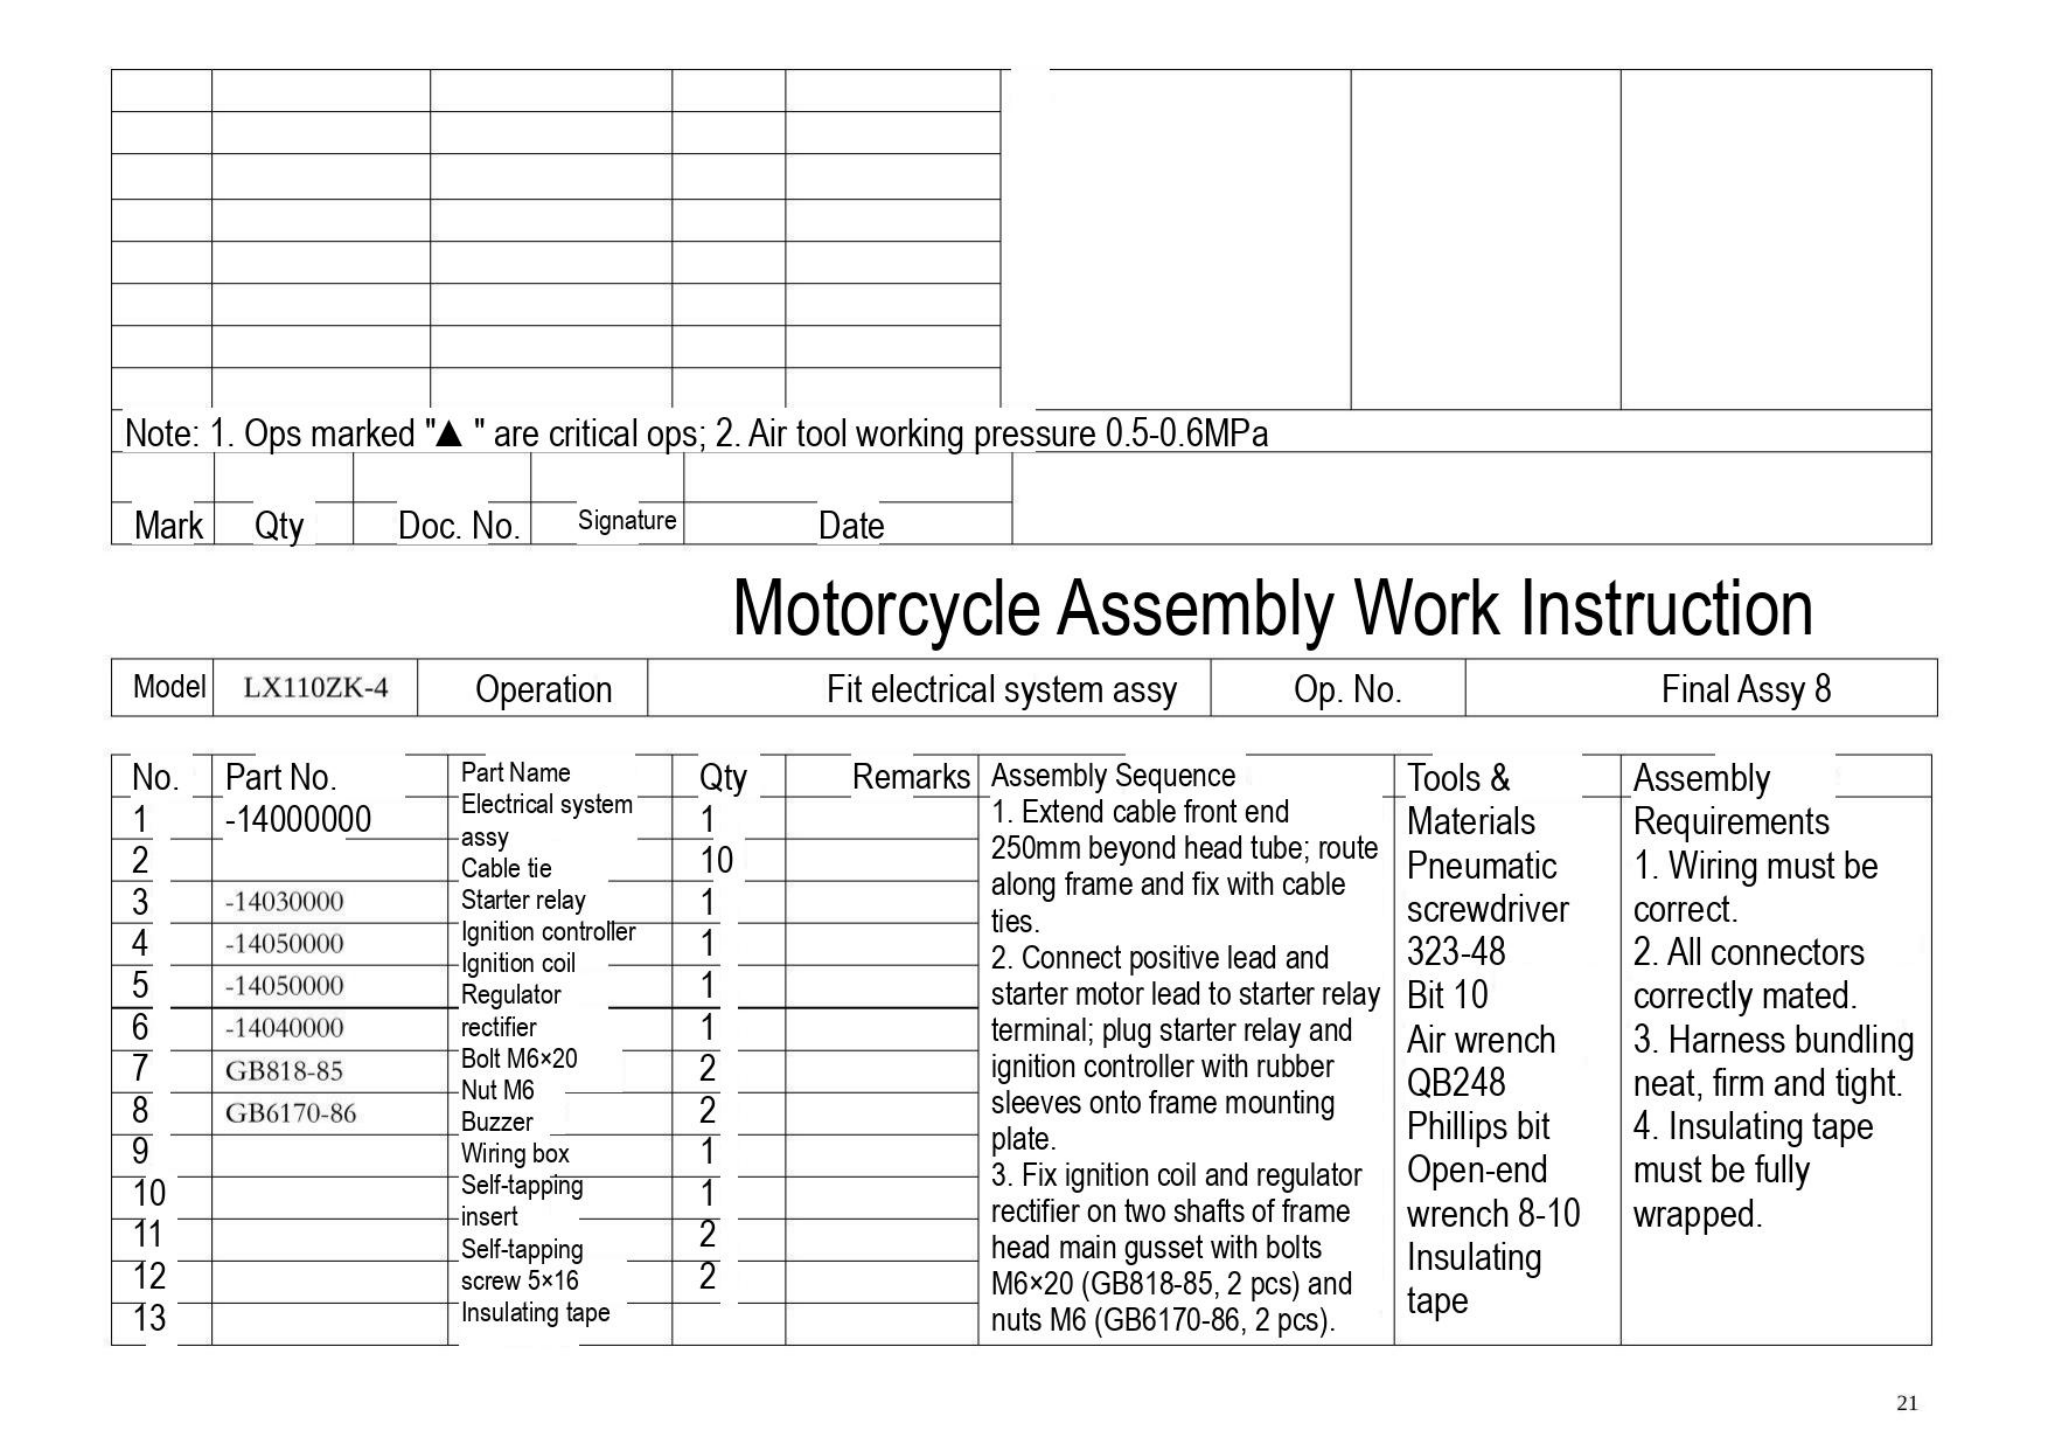Note: 1. Ops marked "▲ " are critical ops; 2. Air tool working pressure 0.5-0.6MPa

| Mark | Qty | Doc. No. | Signature | Date |
|---|---|---|---|---|

# Motorcycle Assembly Work Instruction

| Model | LX110ZK-4 | Operation | Fit electrical system assy | Op. No. | Final Assy 8 |
|---|---|---|---|---|---|

| No. | Part No. | Part Name | Qty | Remarks |
|---|---|---|---|---|
| 1 | -14000000 | Electrical system assy | 1 | |
| 2 | | Cable tie | 10 | |
| 3 | -14030000 | Starter relay | 1 | |
| 4 | -14050000 | Ignition controller | 1 | |
| 5 | -14050000 | Ignition coil | 1 | |
| 6 | -14040000 | Regulator rectifier | 1 | |
| 7 | GB818-85 | Bolt M6×20 | 2 | |
| 8 | GB6170-86 | Nut M6 | 2 | |
| 9 | | Buzzer | 1 | |
| 10 | | Wiring box | 1 | |
| 11 | | Self-tapping insert | 2 | |
| 12 | | Self-tapping screw 5×16 | 2 | |
| 13 | | Insulating tape | | |

Assembly Sequence
1. Extend cable front end 250mm beyond head tube; route along frame and fix with cable ties.
2. Connect positive lead and starter motor lead to starter relay terminal; plug starter relay and ignition controller with rubber sleeves onto frame mounting plate.
3. Fix ignition coil and regulator rectifier on two shafts of frame head main gusset with bolts M6×20 (GB818-85, 2 pcs) and nuts M6 (GB6170-86, 2 pcs).

Tools & Materials
Pneumatic screwdriver 323-48
Bit 10
Air wrench QB248
Phillips bit
Open-end wrench 8-10
Insulating tape

Assembly Requirements
1. Wiring must be correct.
2. All connectors correctly mated.
3. Harness bundling neat, firm and tight.
4. Insulating tape must be fully wrapped.

21
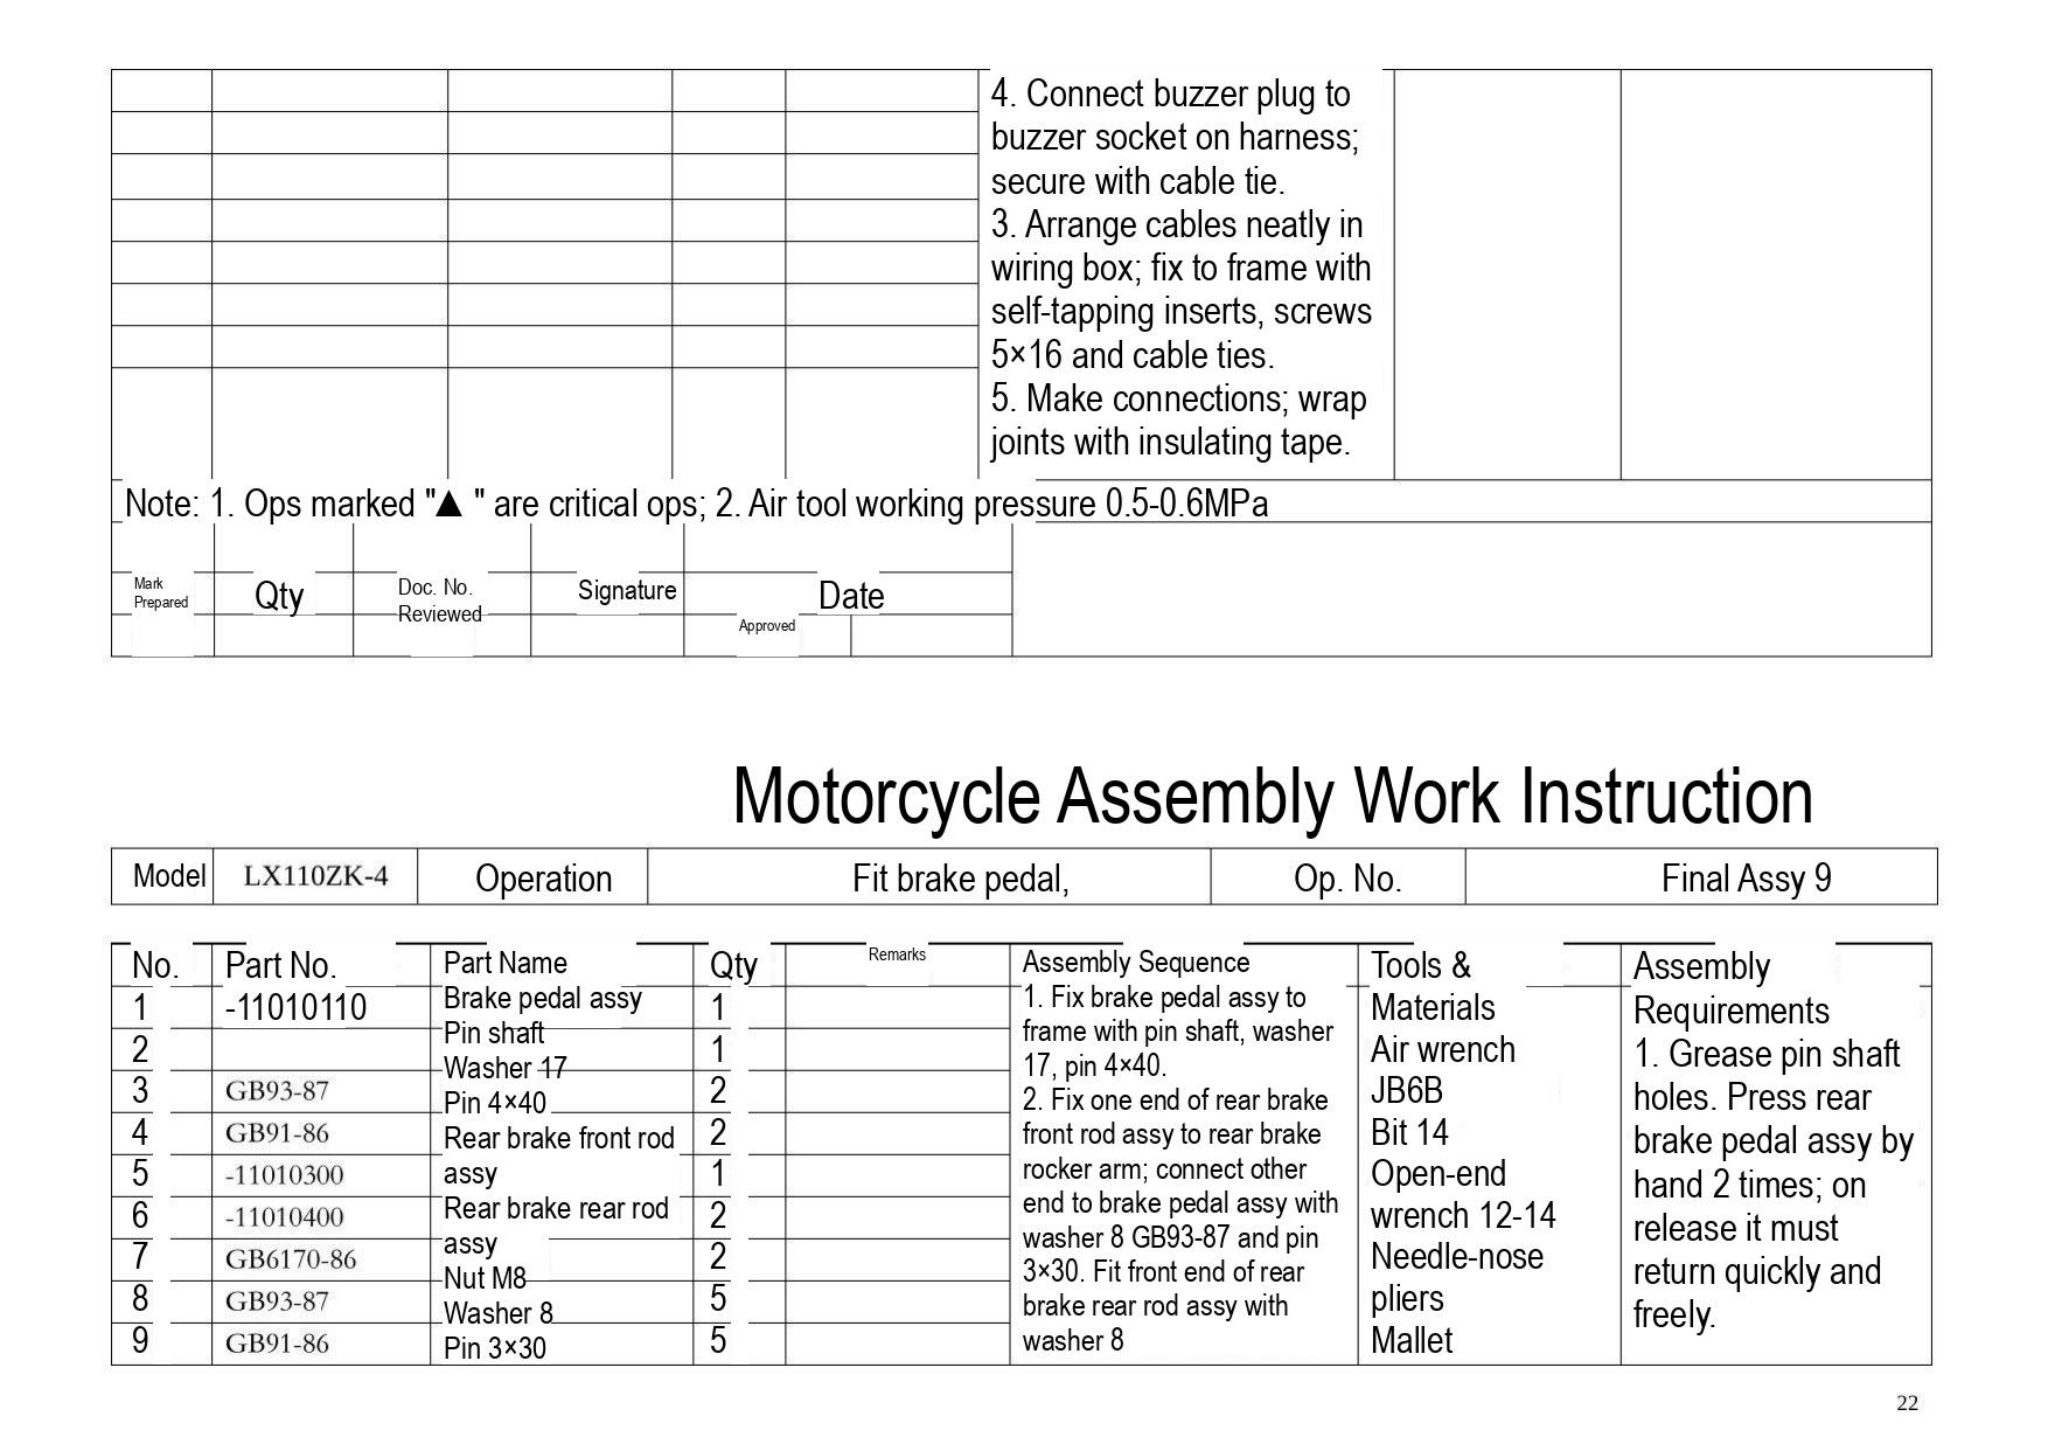4. Connect buzzer plug to buzzer socket on harness; secure with cable tie.
3. Arrange cables neatly in wiring box; fix to frame with self-tapping inserts, screws 5×16 and cable ties.
5. Make connections; wrap joints with insulating tape.

Note: 1. Ops marked "▲ " are critical ops; 2. Air tool working pressure 0.5-0.6MPa

| Mark Prepared | Qty | Doc. No. Reviewed | Signature | Approved | Date |
|---|---|---|---|---|---|

# Motorcycle Assembly Work Instruction

| Model | LX110ZK-4 | Operation | Fit brake pedal, | Op. No. | Final Assy 9 |
|---|---|---|---|---|---|

| No. | Part No. | Part Name | Qty | Remarks |
|---|---|---|---|---|
| 1 | -11010110 | Brake pedal assy | 1 | |
| 2 | | Pin shaft | 1 | |
| 3 | GB93-87 | Washer 17 | 2 | |
| 4 | GB91-86 | Pin 4×40 | 2 | |
| 5 | -11010300 | Rear brake front rod assy | 1 | |
| 6 | -11010400 | Rear brake rear rod assy | 2 | |
| 7 | GB6170-86 | Nut M8 | 2 | |
| 8 | GB93-87 | Washer 8 | 5 | |
| 9 | GB91-86 | Pin 3×30 | 5 | |

Assembly Sequence
1. Fix brake pedal assy to frame with pin shaft, washer 17, pin 4×40.
2. Fix one end of rear brake front rod assy to rear brake rocker arm; connect other end to brake pedal assy with washer 8 GB93-87 and pin 3×30. Fit front end of rear brake rear rod assy with washer 8

Tools & Materials
Air wrench
JB6B
Bit 14
Open-end wrench 12-14
Needle-nose pliers
Mallet

Assembly Requirements
1. Grease pin shaft holes. Press rear brake pedal assy by hand 2 times; on release it must return quickly and freely.

22
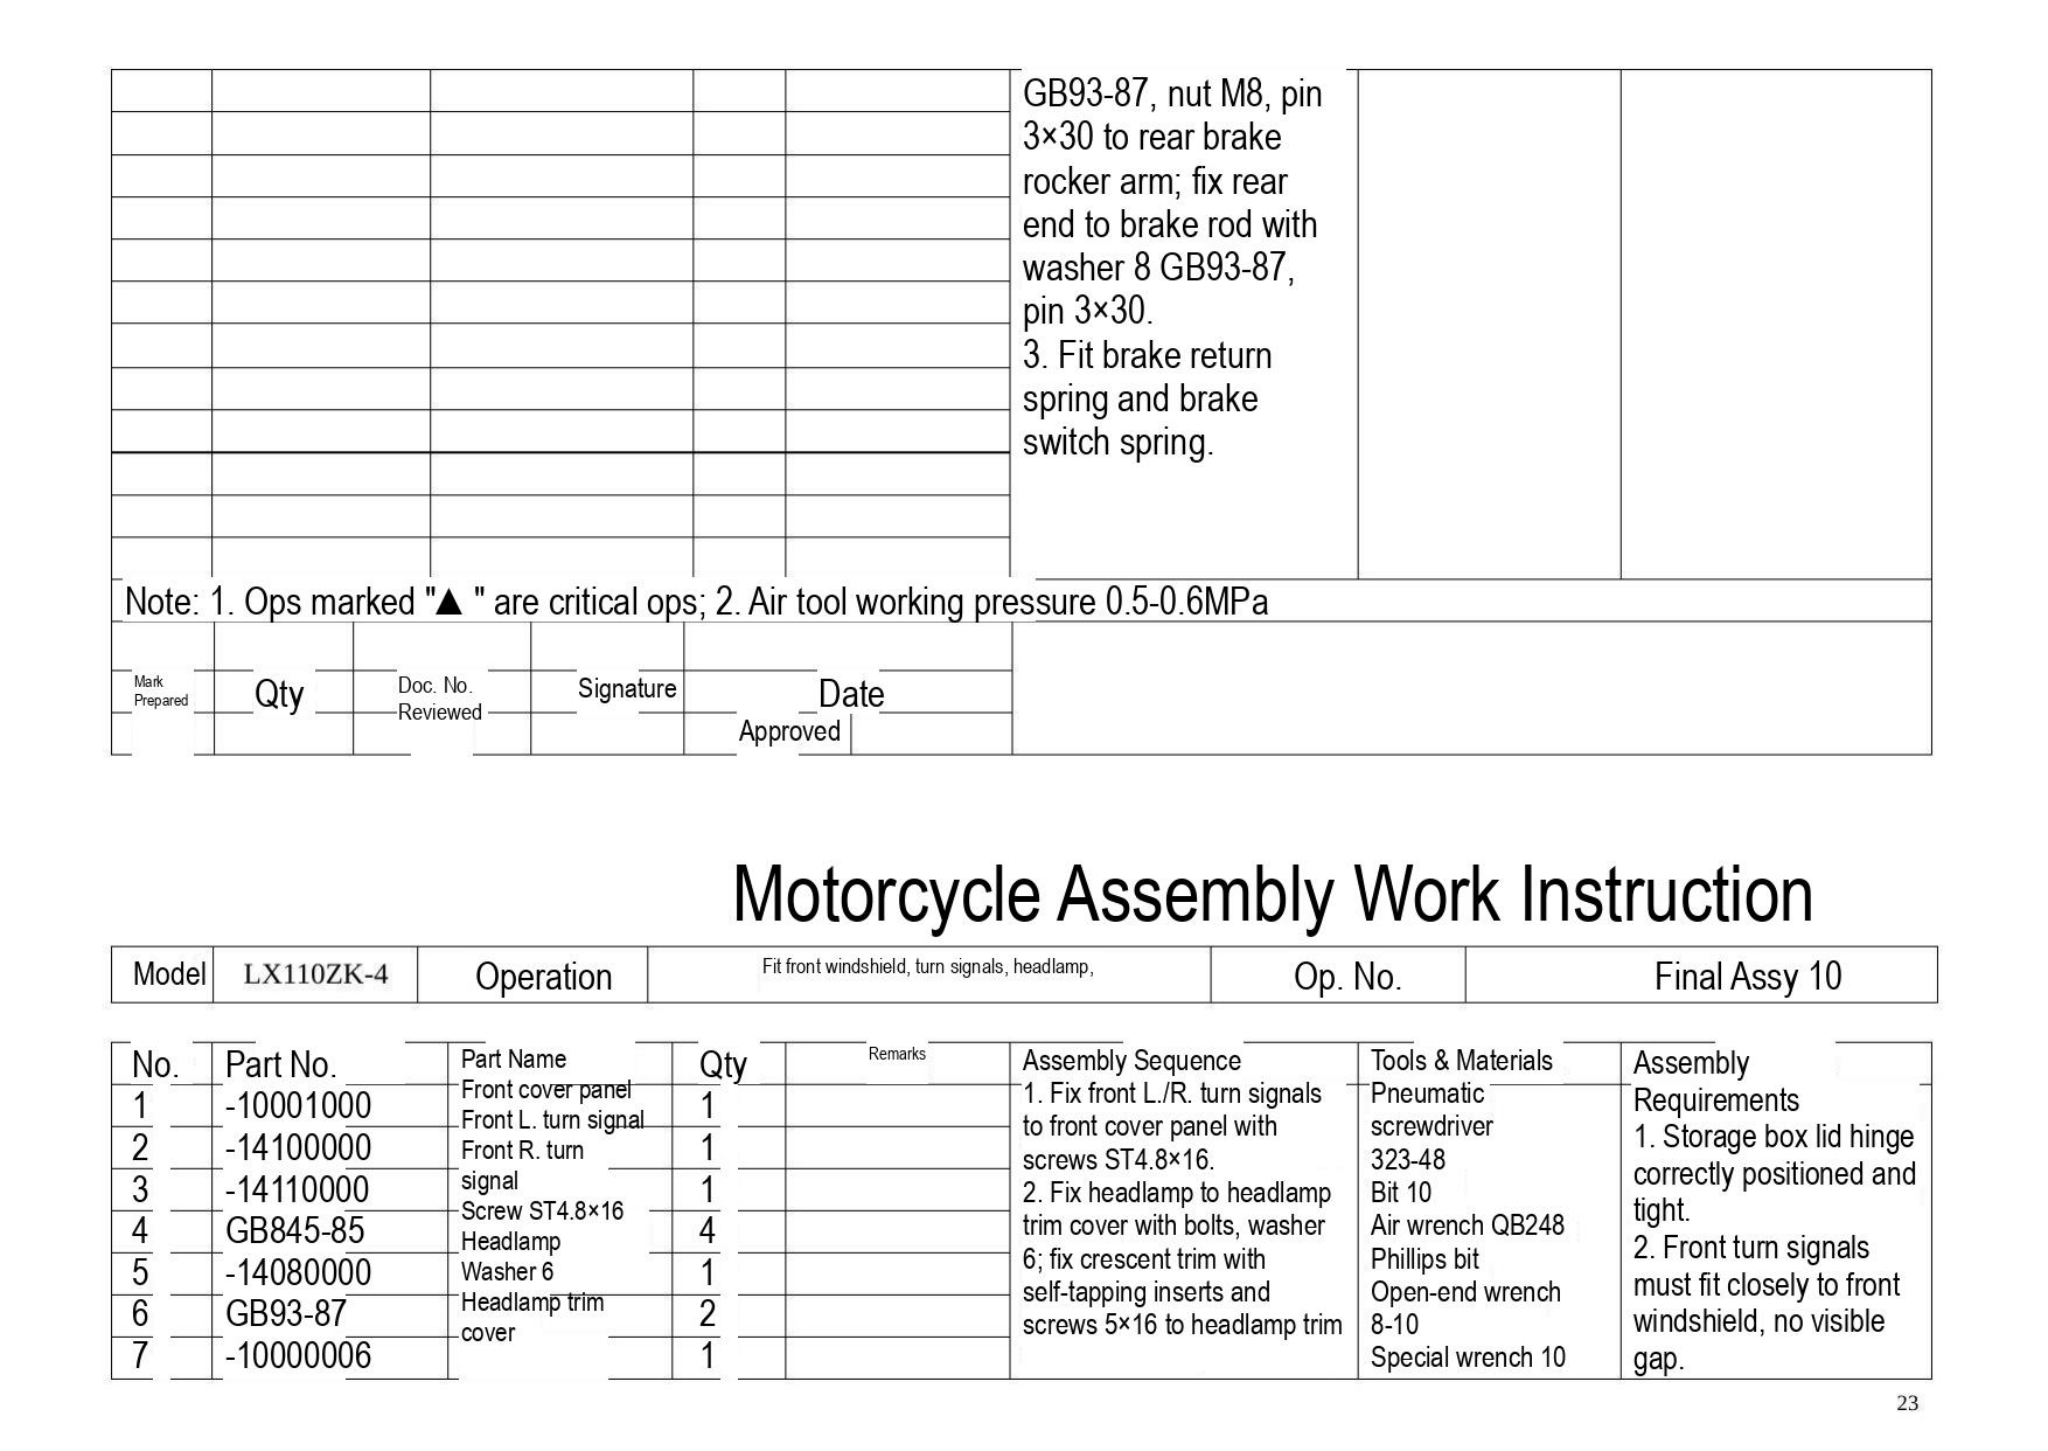| | | | | | | | |
|---|---|---|---|---|---|---|---|
| | | | | | GB93-87, nut M8, pin 3×30 to rear brake rocker arm; fix rear end to brake rod with washer 8 GB93-87, pin 3×30.<br>3. Fit brake return spring and brake switch spring. | | |

Note: 1. Ops marked "▲ " are critical ops; 2. Air tool working pressure 0.5-0.6MPa

| Mark Prepared | Qty | Doc. No. Reviewed | Signature | Date Approved | |
|---|---|---|---|---|---|

# Motorcycle Assembly Work Instruction

| Model | LX110ZK-4 | Operation | Fit front windshield, turn signals, headlamp, | Op. No. | Final Assy 10 |
|---|---|---|---|---|---|

| No. | Part No. | Part Name | Qty | Remarks | Assembly Sequence | Tools & Materials | Assembly Requirements |
|---|---|---|---|---|---|---|---|
| 1 | -10001000 | Front cover panel | 1 | | 1. Fix front L./R. turn signals to front cover panel with screws ST4.8×16.<br>2. Fix headlamp to headlamp trim cover with bolts, washer 6; fix crescent trim with self-tapping inserts and screws 5×16 to headlamp trim | Pneumatic screwdriver 323-48<br>Bit 10<br>Air wrench QB248<br>Phillips bit<br>Open-end wrench 8-10<br>Special wrench 10 | 1. Storage box lid hinge correctly positioned and tight.<br>2. Front turn signals must fit closely to front windshield, no visible gap. |
| 2 | -14100000 | Front L. turn signal | 1 | | | | |
| 3 | -14110000 | Front R. turn signal | 1 | | | | |
| 4 | GB845-85 | Screw ST4.8×16 | 4 | | | | |
| 5 | -14080000 | Headlamp | 1 | | | | |
| 6 | GB93-87 | Washer 6 | 2 | | | | |
| 7 | -10000006 | Headlamp trim cover | 1 | | | | |

23
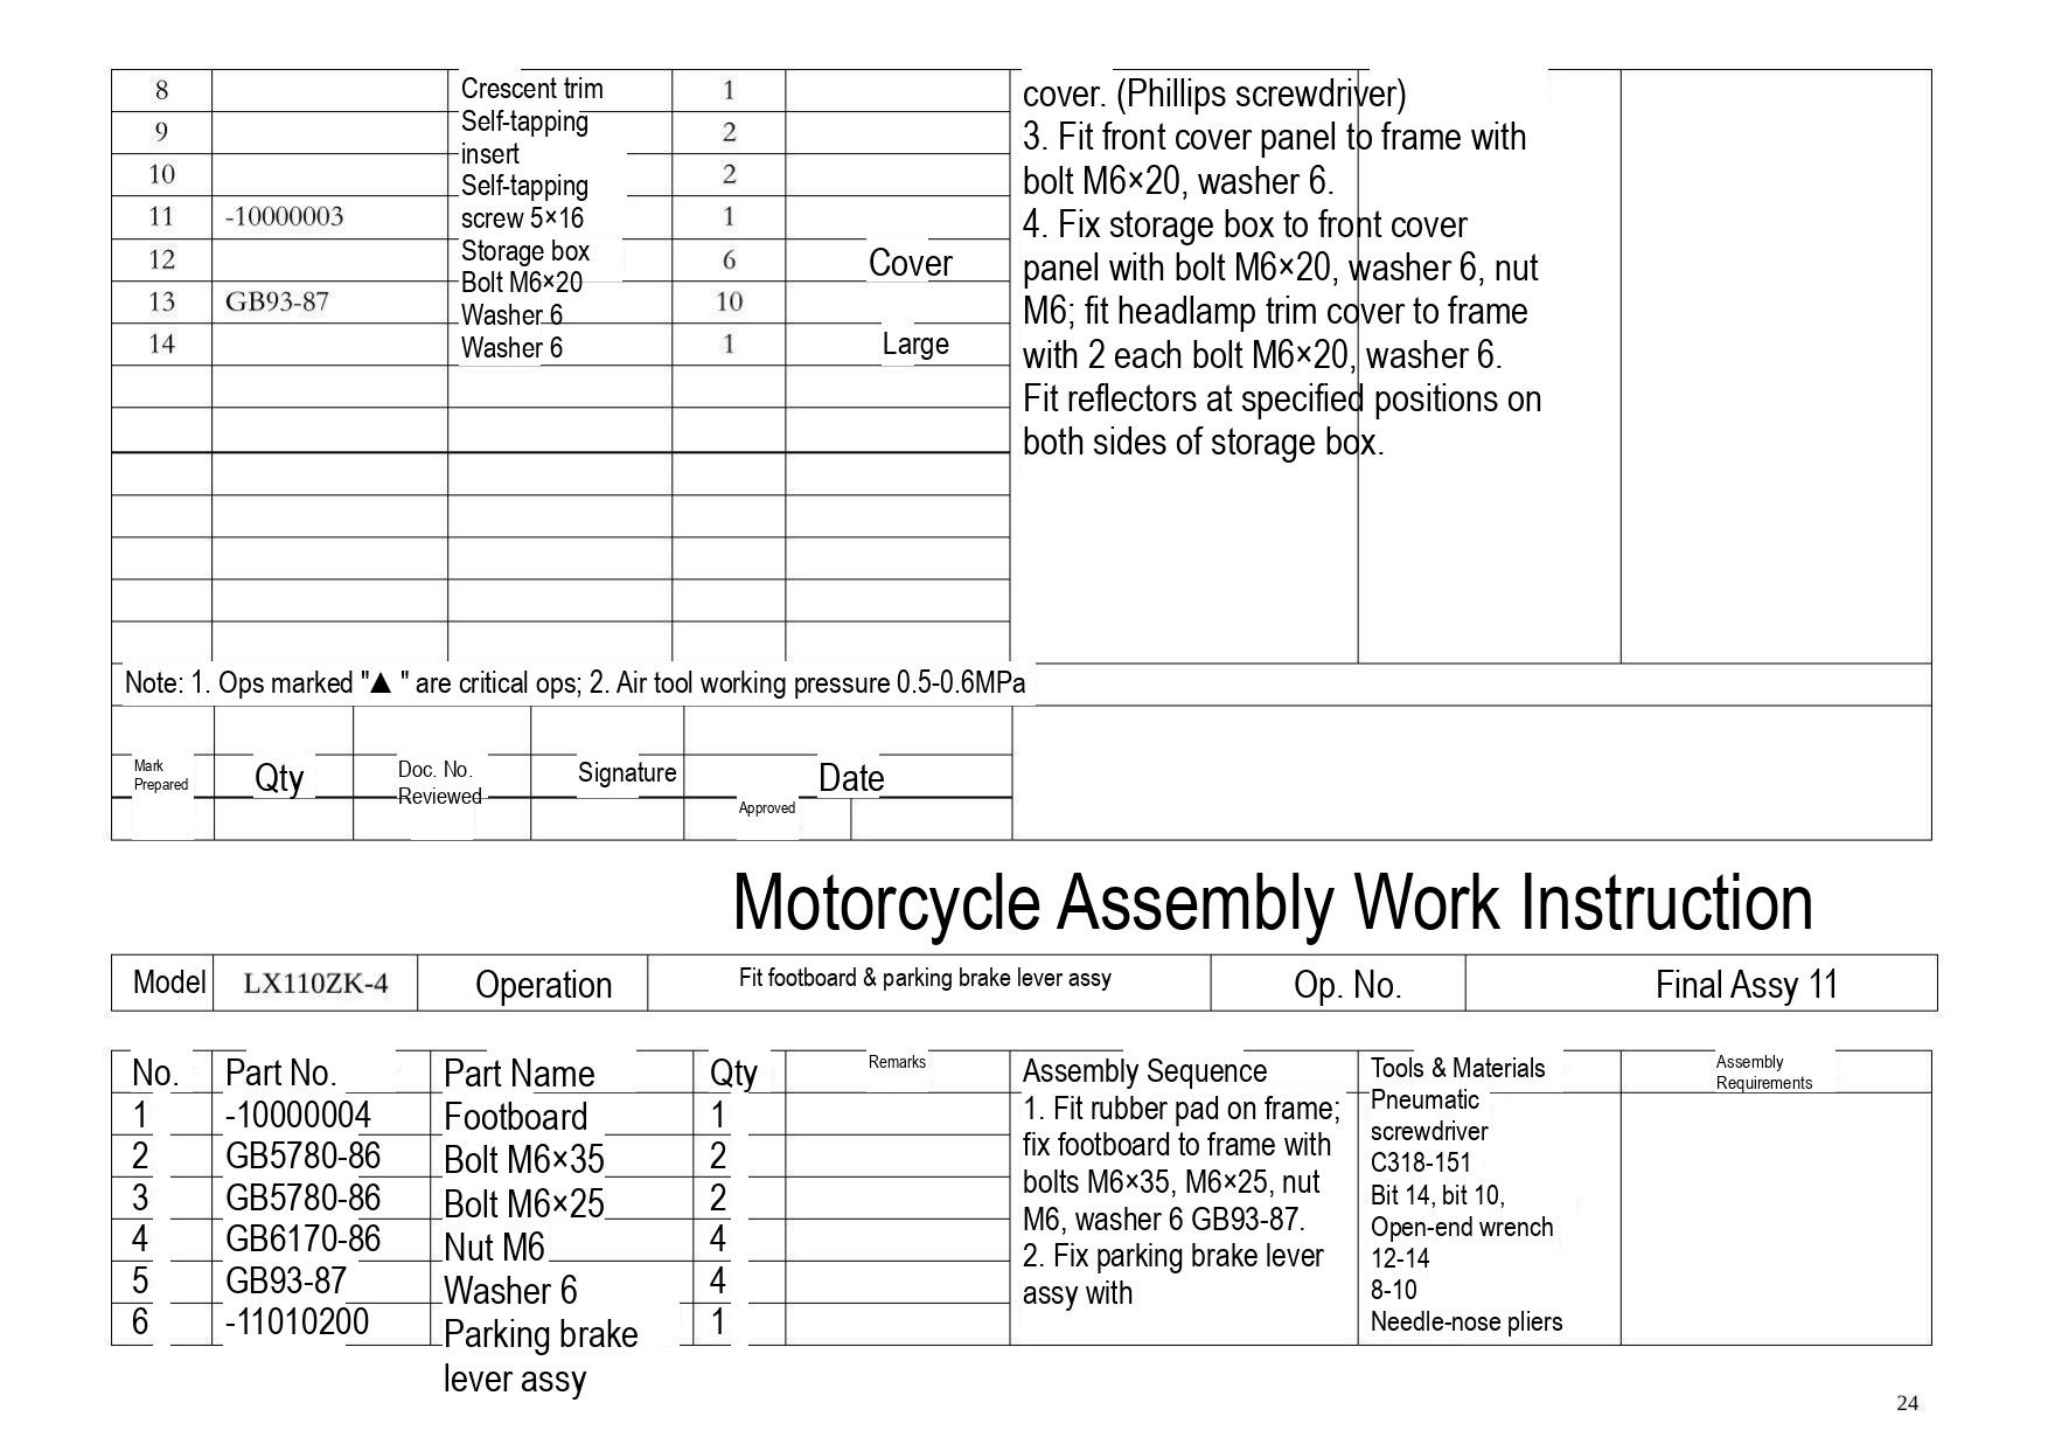| 8 | | Crescent trim | 1 | | cover. (Phillips screwdriver) 3. Fit front cover panel to frame with bolt M6×20, washer 6. 4. Fix storage box to front cover panel with bolt M6×20, washer 6, nut M6; fit headlamp trim cover to frame with 2 each bolt M6×20, washer 6. Fit reflectors at specified positions on both sides of storage box. | | |
|---|---|---|---|---|---|---|---|
| 9 | | Self-tapping insert | 2 | | | | |
| 10 | | Self-tapping screw 5×16 | 2 | | | | |
| 11 | -10000003 | Storage box | 1 | | | | |
| 12 | | Bolt M6×20 | 6 | Cover | | | |
| 13 | GB93-87 | Washer 6 | 10 | | | | |
| 14 | | Washer 6 | 1 | Large | | | |

Note: 1. Ops marked "▲ " are critical ops; 2. Air tool working pressure 0.5-0.6MPa

| Mark Prepared | Qty | Doc. No. Reviewed | Signature | Approved | Date |
|---|---|---|---|---|---|
| | | | | | |

# Motorcycle Assembly Work Instruction

| Model | LX110ZK-4 | Operation | Fit footboard & parking brake lever assy | Op. No. | Final Assy 11 |
|---|---|---|---|---|---|

| No. | Part No. | Part Name | Qty | Remarks | Assembly Sequence | Tools & Materials | Assembly Requirements |
|---|---|---|---|---|---|---|---|
| 1 | -10000004 | Footboard | 1 | | 1. Fit rubber pad on frame; fix footboard to frame with bolts M6×35, M6×25, nut M6, washer 6 GB93-87. 2. Fix parking brake lever assy with | Pneumatic screwdriver C318-151 Bit 14, bit 10, Open-end wrench 12-14 8-10 Needle-nose pliers | |
| 2 | GB5780-86 | Bolt M6×35 | 2 | | | | |
| 3 | GB5780-86 | Bolt M6×25 | 2 | | | | |
| 4 | GB6170-86 | Nut M6 | 4 | | | | |
| 5 | GB93-87 | Washer 6 | 4 | | | | |
| 6 | -11010200 | Parking brake lever assy | 1 | | | | |

24
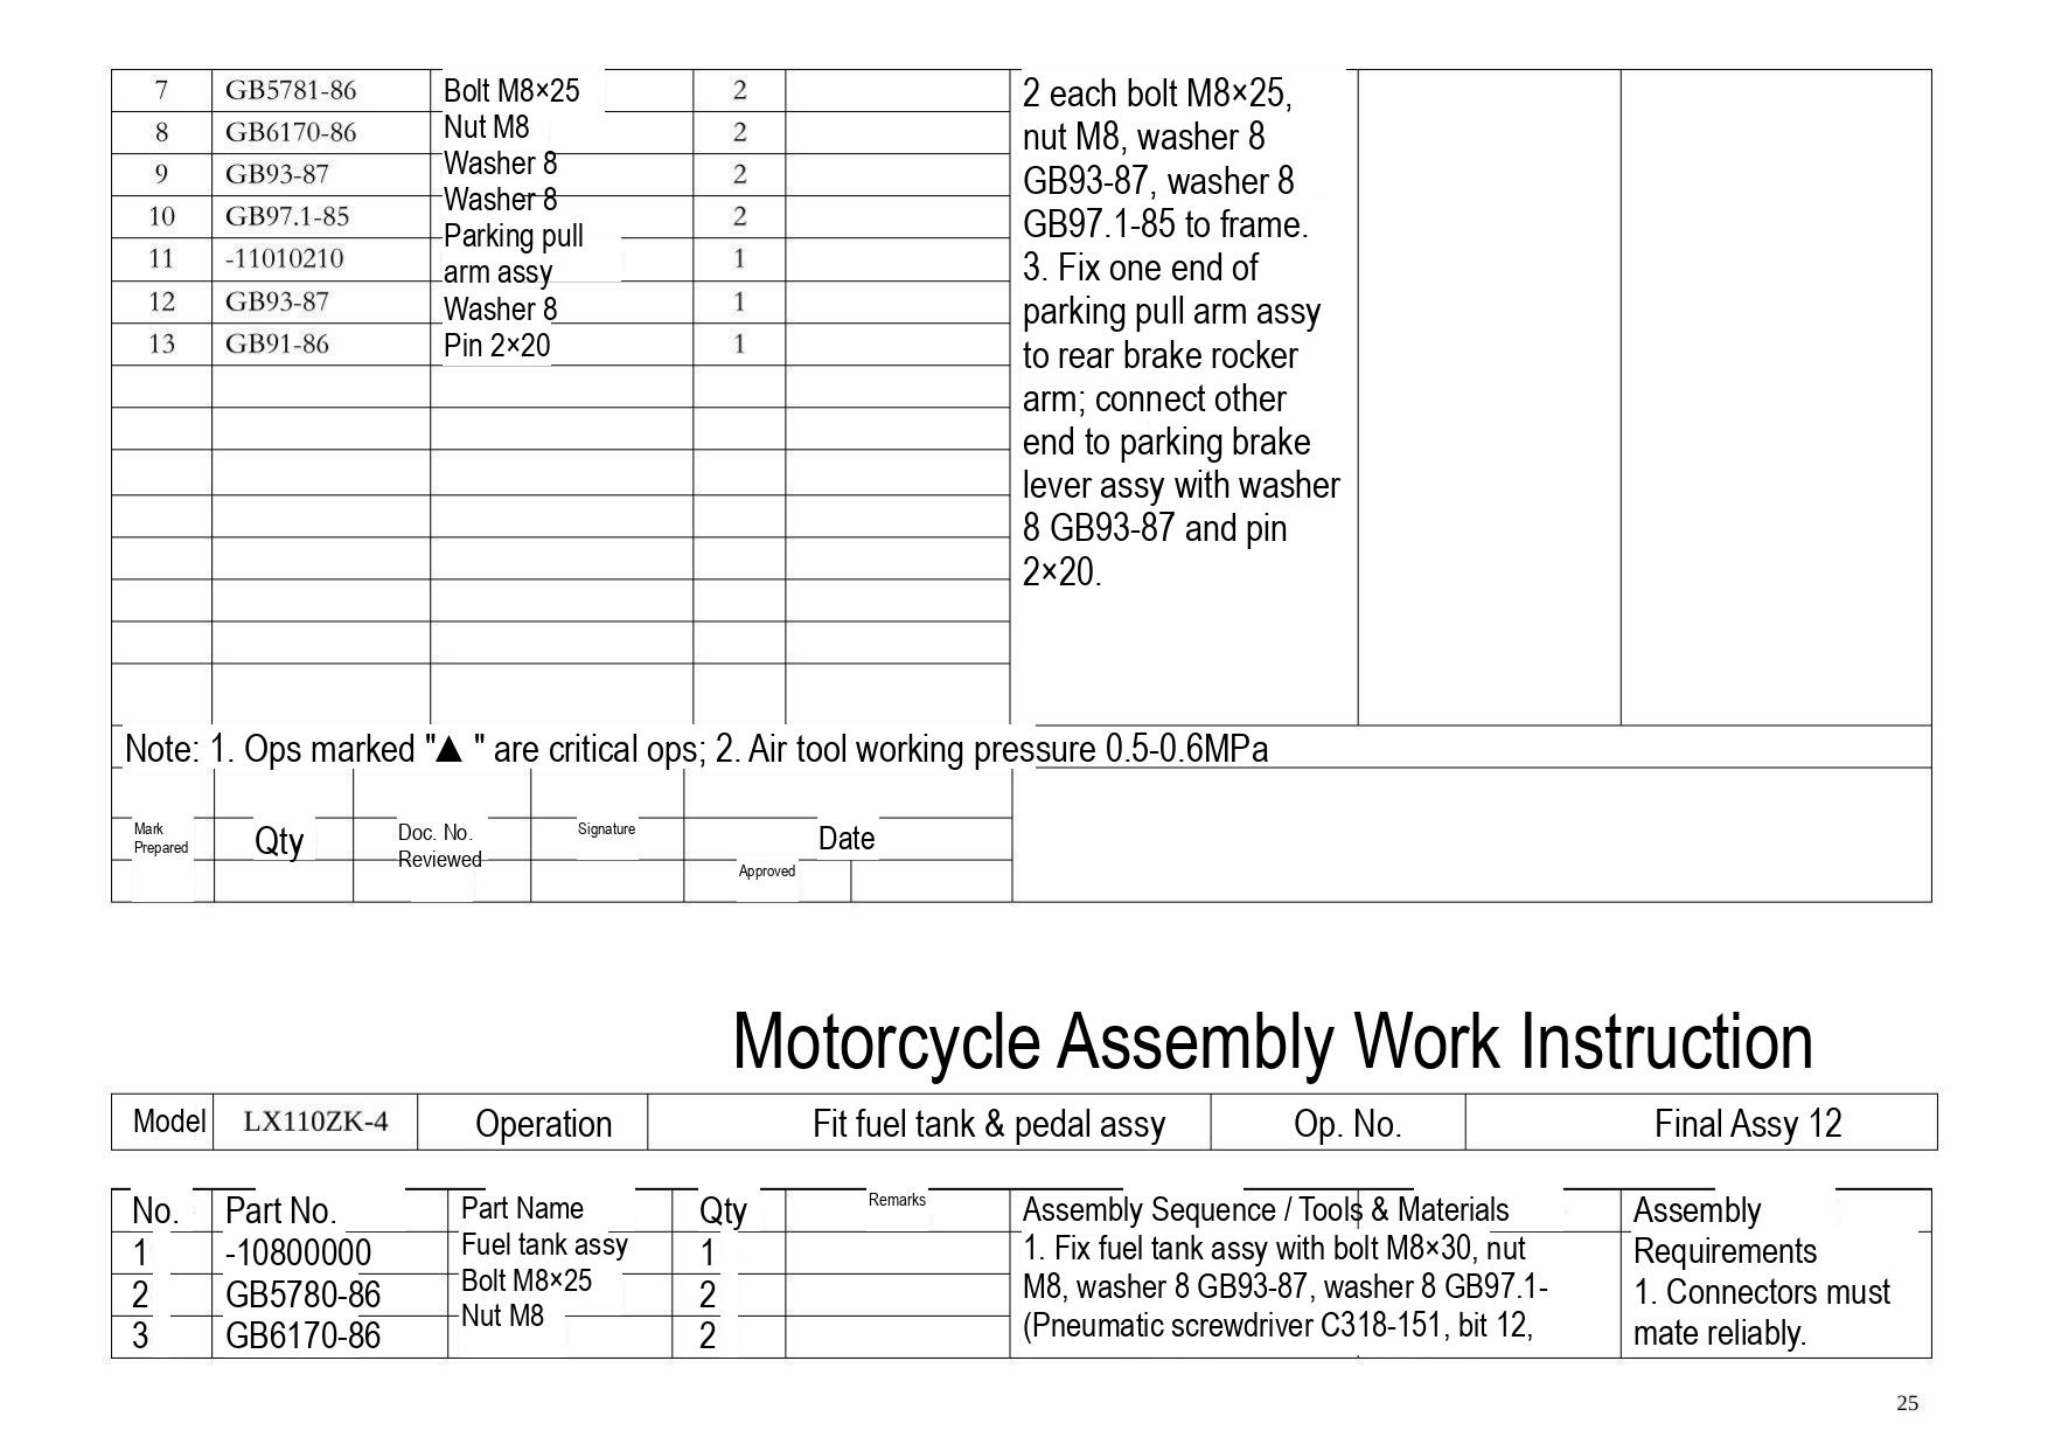| | | | | | | | |
|---|---|---|---|---|---|---|---|
| 7 | GB5781-86 | Bolt M8×25 | 2 | | 2 each bolt M8×25, nut M8, washer 8 GB93-87, washer 8 GB97.1-85 to frame. 3. Fix one end of parking pull arm assy to rear brake rocker arm; connect other end to parking brake lever assy with washer 8 GB93-87 and pin 2×20. | | |
| 8 | GB6170-86 | Nut M8 | 2 | | | | |
| 9 | GB93-87 | Washer 8 | 2 | | | | |
| 10 | GB97.1-85 | Washer 8 | 2 | | | | |
| 11 | -11010210 | Parking pull arm assy | 1 | | | | |
| 12 | GB93-87 | Washer 8 | 1 | | | | |
| 13 | GB91-86 | Pin 2×20 | 1 | | | | |

Note: 1. Ops marked "▲ " are critical ops; 2. Air tool working pressure 0.5-0.6MPa

| Mark Prepared | Qty | Doc. No. Reviewed | Signature | Approved | Date |
|---|---|---|---|---|---|

Motorcycle Assembly Work Instruction

| Model | LX110ZK-4 | Operation | Fit fuel tank & pedal assy | Op. No. | Final Assy 12 |
|---|---|---|---|---|---|

| No. | Part No. | Part Name | Qty | Remarks | Assembly Sequence / Tools & Materials | Assembly Requirements |
|---|---|---|---|---|---|---|
| 1 | -10800000 | Fuel tank assy | 1 | | 1. Fix fuel tank assy with bolt M8×30, nut M8, washer 8 GB93-87, washer 8 GB97.1- (Pneumatic screwdriver C318-151, bit 12, | 1. Connectors must mate reliably. |
| 2 | GB5780-86 | Bolt M8×25 | 2 | | | |
| 3 | GB6170-86 | Nut M8 | 2 | | | |

25
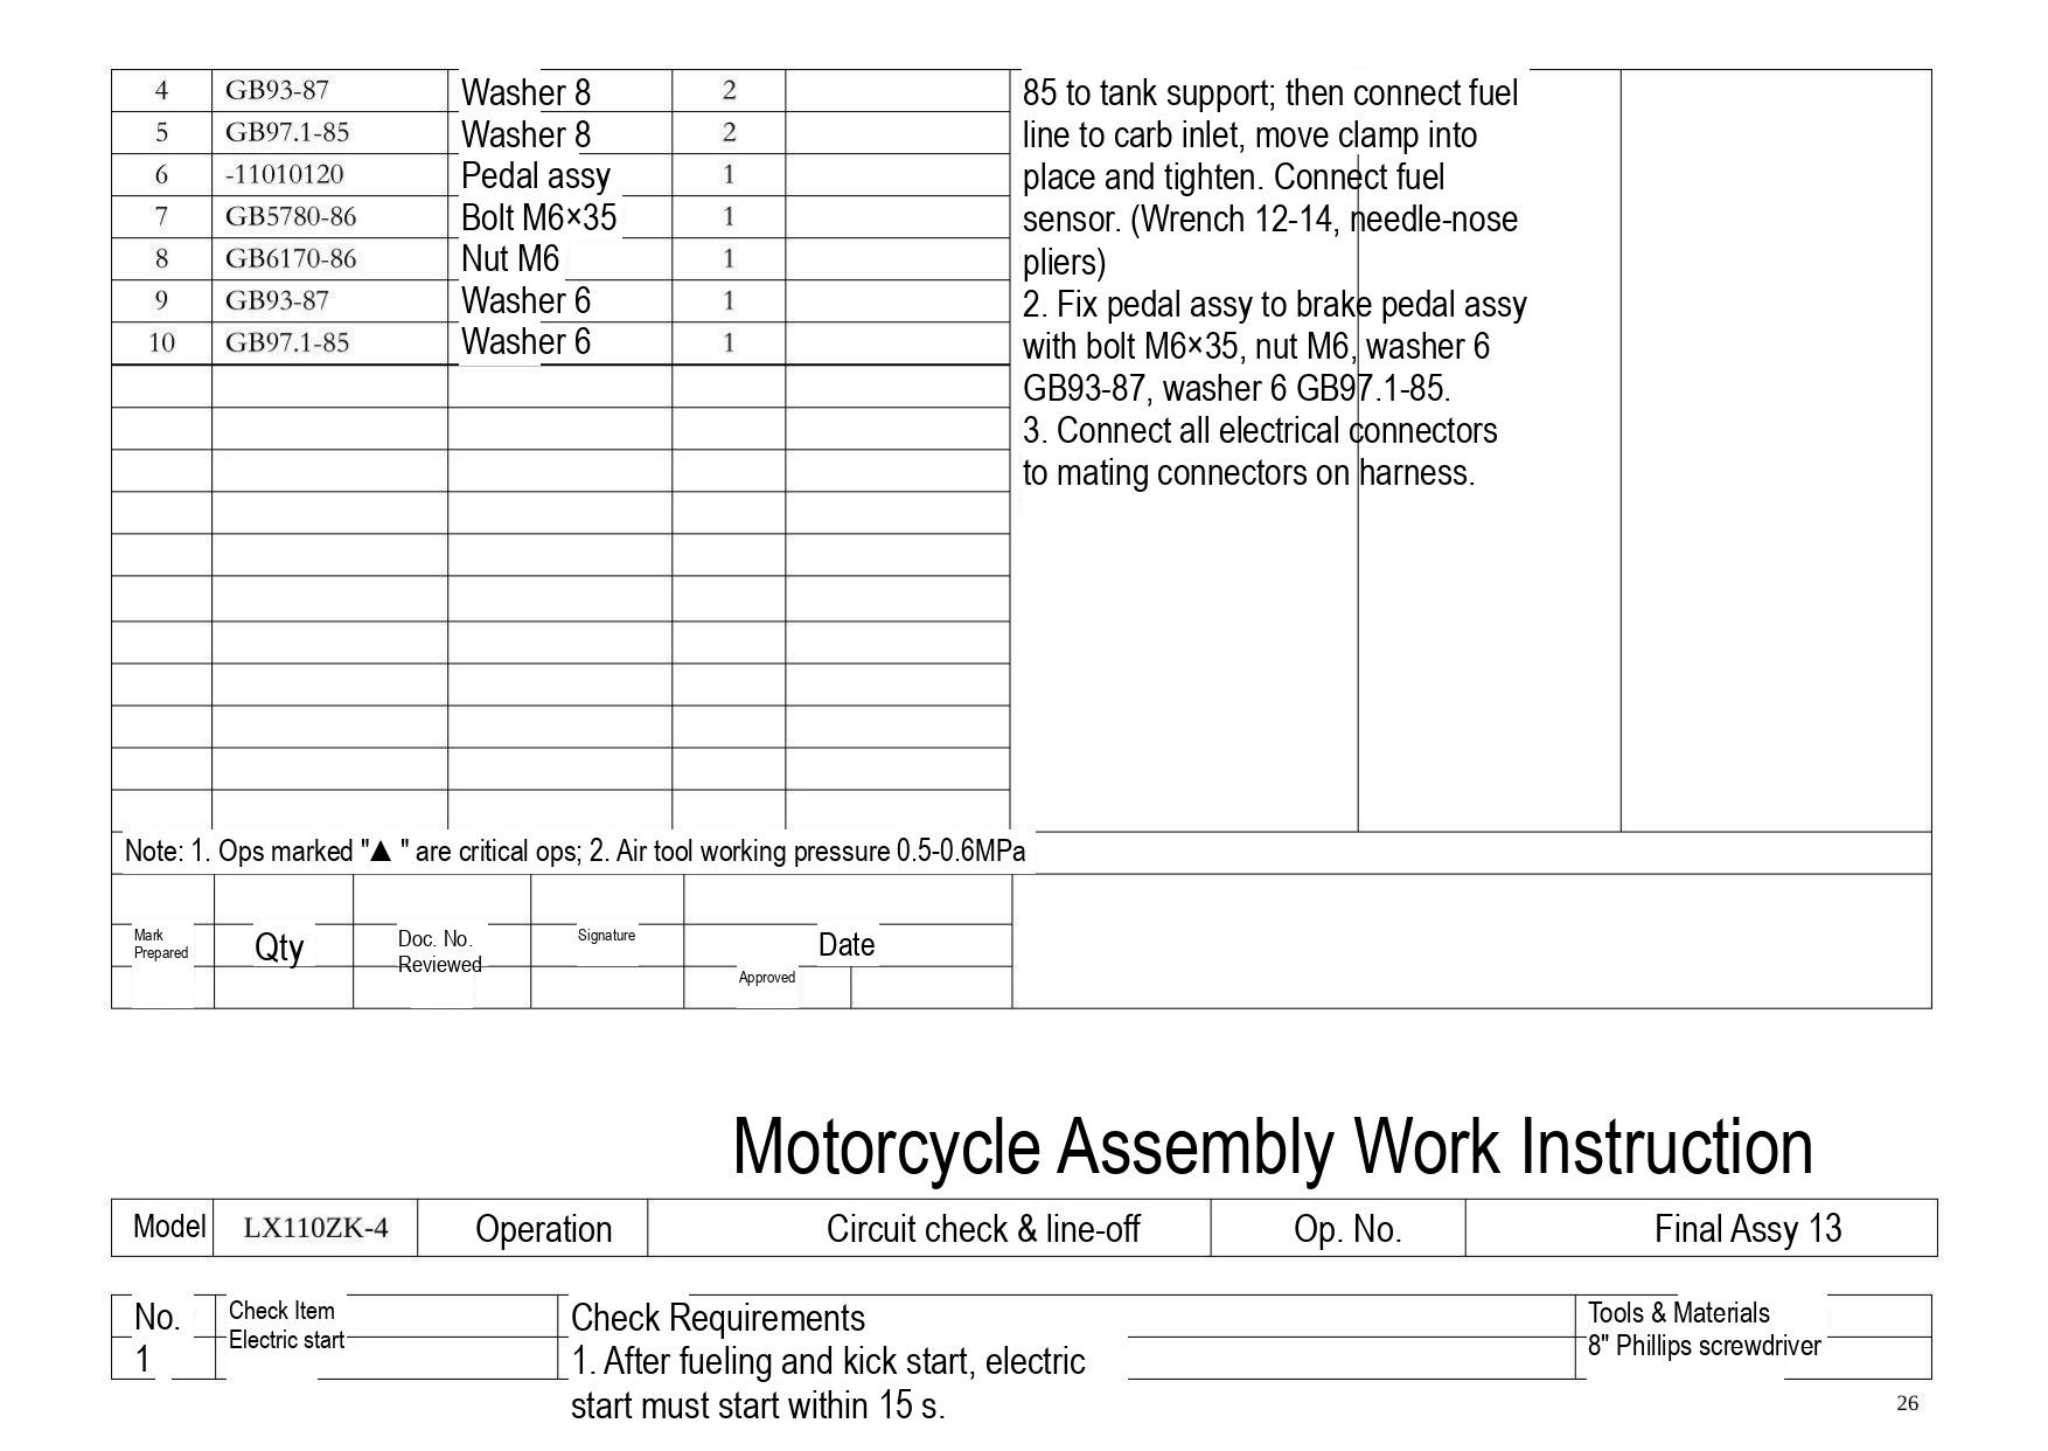| 4 | GB93-87 | Washer 8 | 2 |  |
|---|---|---|---|---|
| 5 | GB97.1-85 | Washer 8 | 2 |  |
| 6 | -11010120 | Pedal assy | 1 |  |
| 7 | GB5780-86 | Bolt M6×35 | 1 |  |
| 8 | GB6170-86 | Nut M6 | 1 |  |
| 9 | GB93-87 | Washer 6 | 1 |  |
| 10 | GB97.1-85 | Washer 6 | 1 |  |

85 to tank support; then connect fuel line to carb inlet, move clamp into place and tighten. Connect fuel sensor. (Wrench 12-14, needle-nose pliers)
2. Fix pedal assy to brake pedal assy with bolt M6×35, nut M6, washer 6 GB93-87, washer 6 GB97.1-85.
3. Connect all electrical connectors to mating connectors on harness.

Note: 1. Ops marked "▲ " are critical ops; 2. Air tool working pressure 0.5-0.6MPa

| Mark<br>Prepared | Qty | Doc. No.<br>Reviewed | Signature | Approved | Date |
|---|---|---|---|---|---|

# Motorcycle Assembly Work Instruction

| Model | LX110ZK-4 | Operation | Circuit check & line-off | Op. No. | Final Assy 13 |
|---|---|---|---|---|---|

| No. | Check Item | Check Requirements | Tools & Materials |
|---|---|---|---|
| 1 | Electric start | 1. After fueling and kick start, electric start must start within 15 s. | 8" Phillips screwdriver |

26
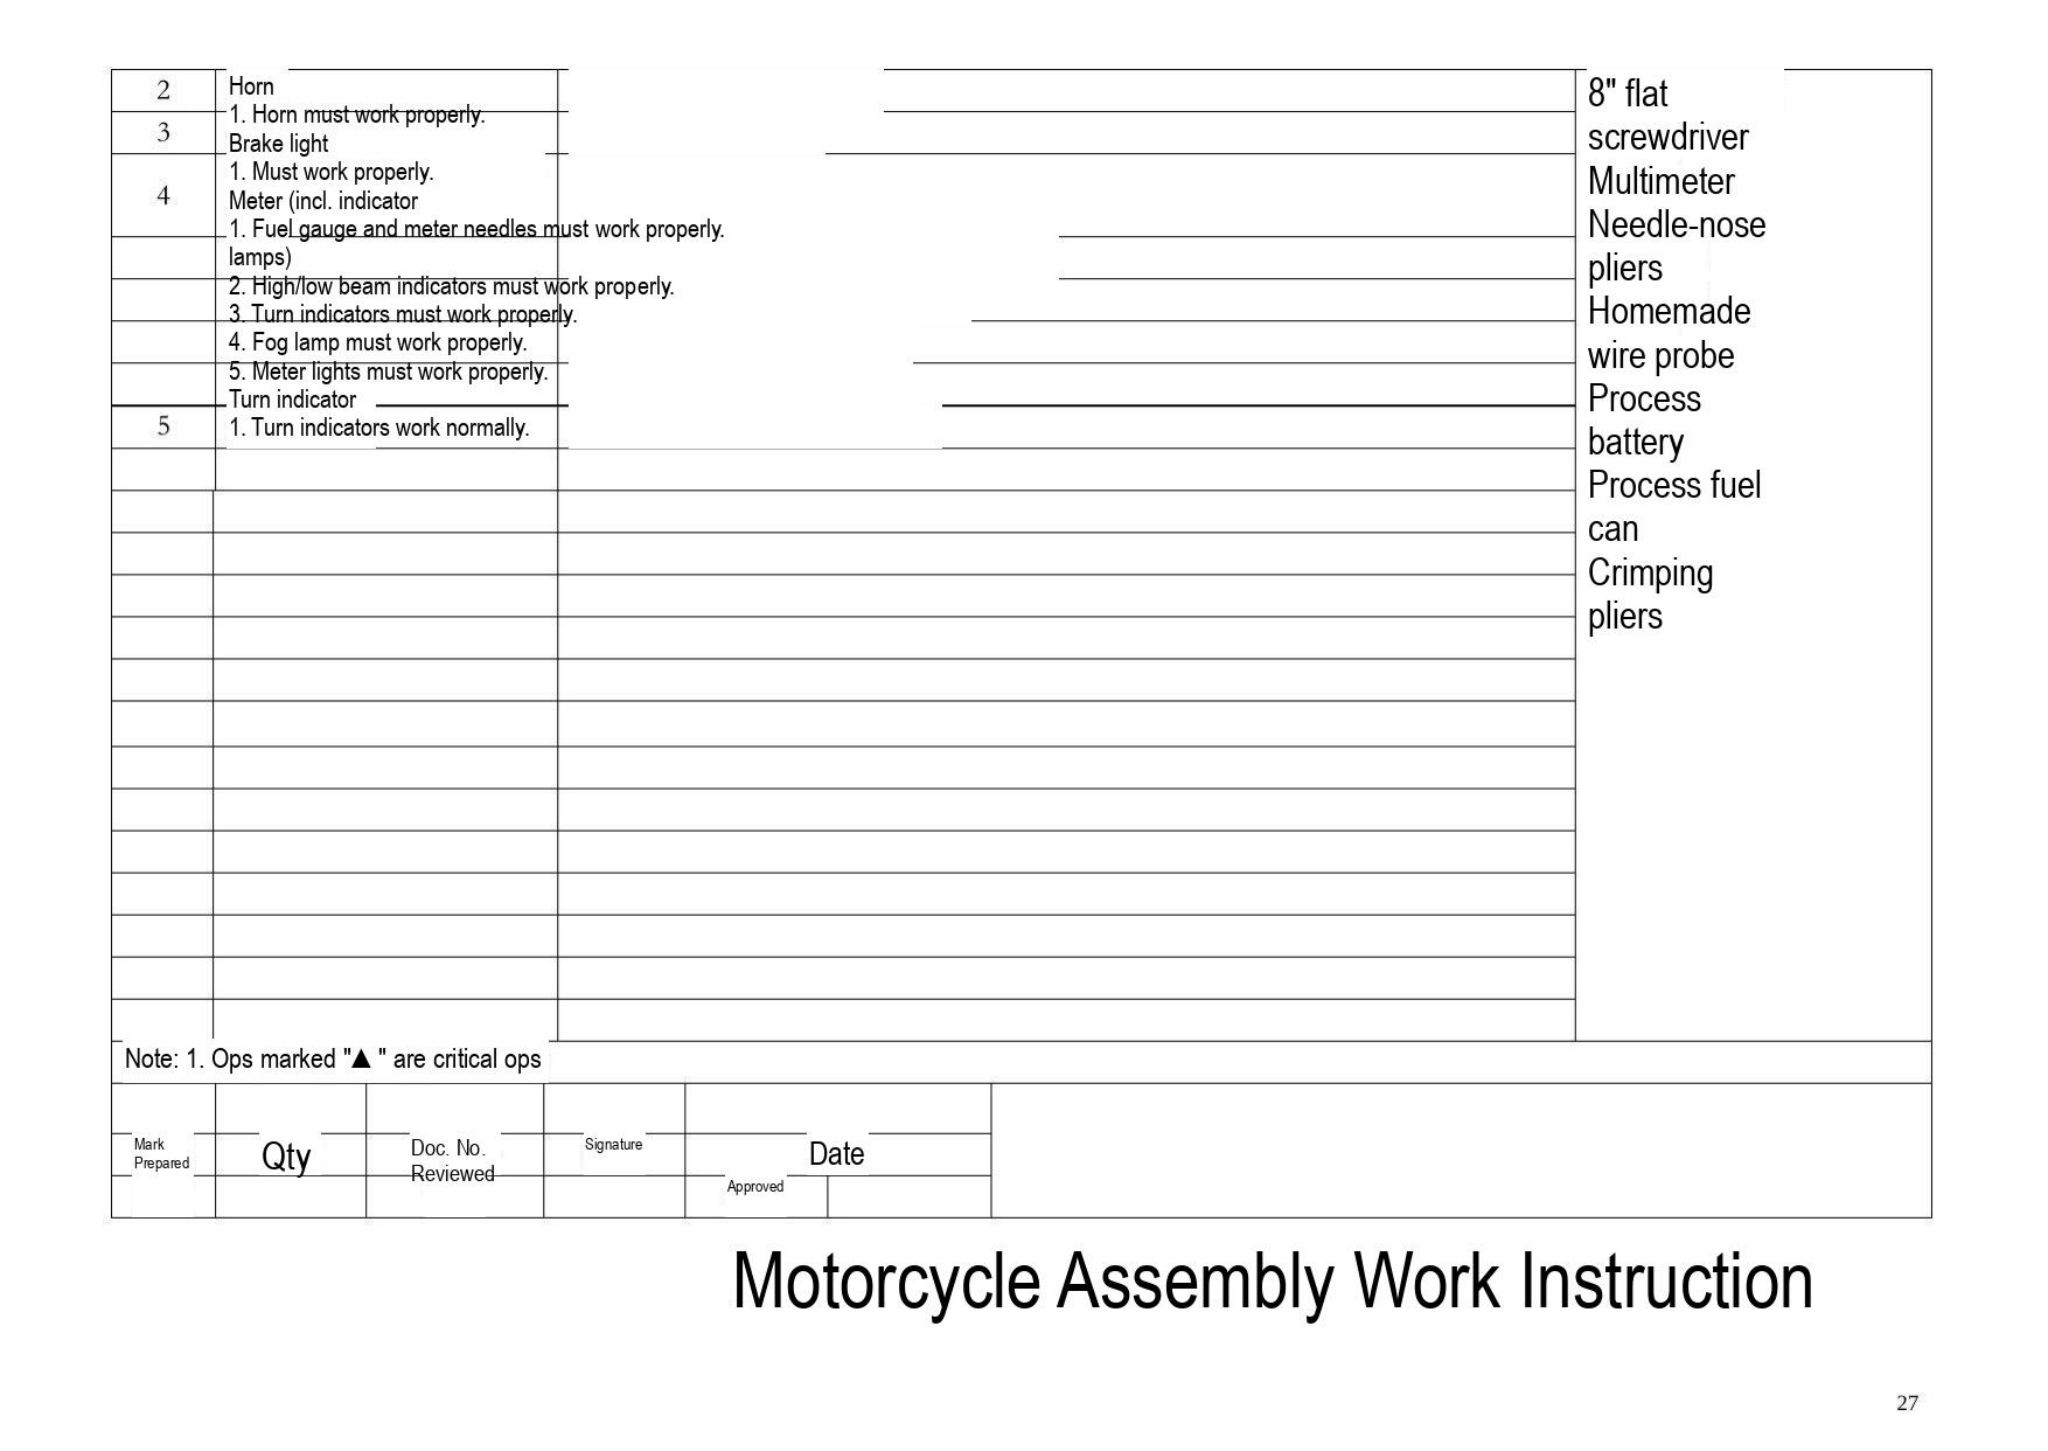| | | | |
|---|---|---|---|
| 2 | Horn<br>1. Horn must work properly. | | 8" flat screwdriver<br>Multimeter<br>Needle-nose pliers<br>Homemade wire probe<br>Process battery<br>Process fuel can<br>Crimping pliers |
| 3 | Brake light<br>1. Must work properly. | | |
| 4 | Meter (incl. indicator<br>1. Fuel gauge and meter needles must work properly.<br>lamps)<br>2. High/low beam indicators must work properly.<br>3. Turn indicators must work properly.<br>4. Fog lamp must work properly.<br>5. Meter lights must work properly. | | |
| 5 | Turn indicator<br>1. Turn indicators work normally. | | |

Note: 1. Ops marked "▲ " are critical ops

| Mark<br>Prepared | Qty | Doc. No.<br>Reviewed | Signature | Date<br>Approved | |
|---|---|---|---|---|---|
| | | | | | |

Motorcycle Assembly Work Instruction

27